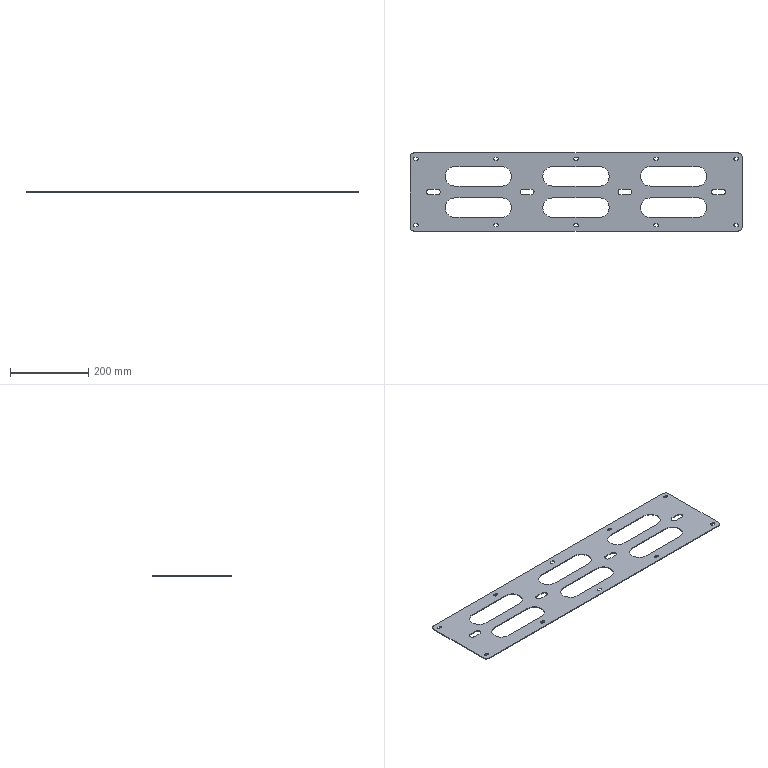Part | SolidWorks | features BaseBody 1 | 1 solid | 110 faces | box 850 x 200 x 2 mm | volume 238983 mm3 | cylinder 64 | plane 46 | commonest cylinder face diameters 7 x30 50 x18 15 x12 20 x4